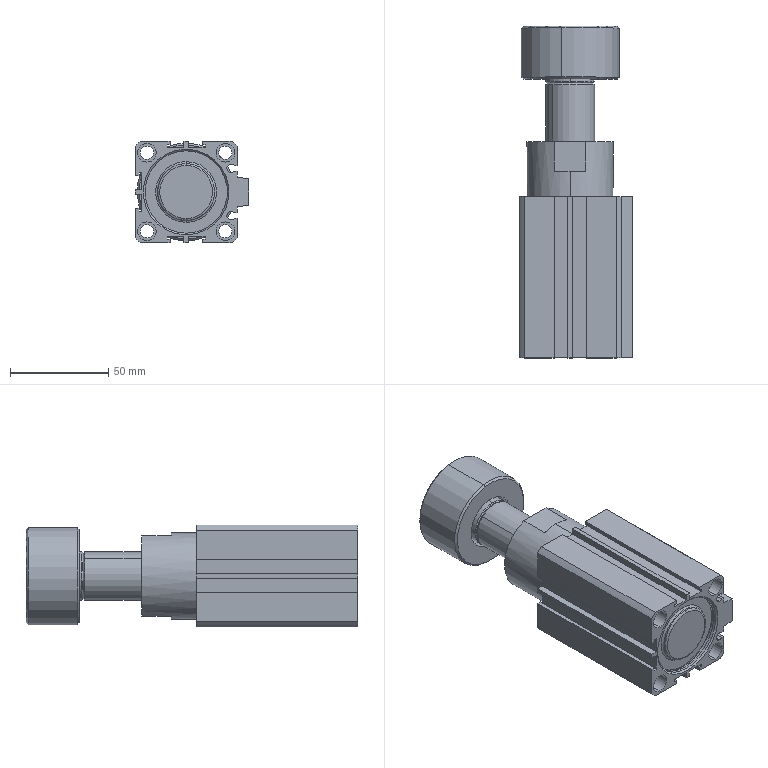Part | SolidWorks | 6 solids | 296 faces | box 58 x 169.2 x 52 mm | volume 267597 mm3 | cylinder 92 | plane 91 | torus 53 | cone 28 | sphere 28 | spline 4 | commonest cylinder face diameters 9.5 x16 6.8 x10 25 x8 4.4 x6 29 x6 2.2 x4